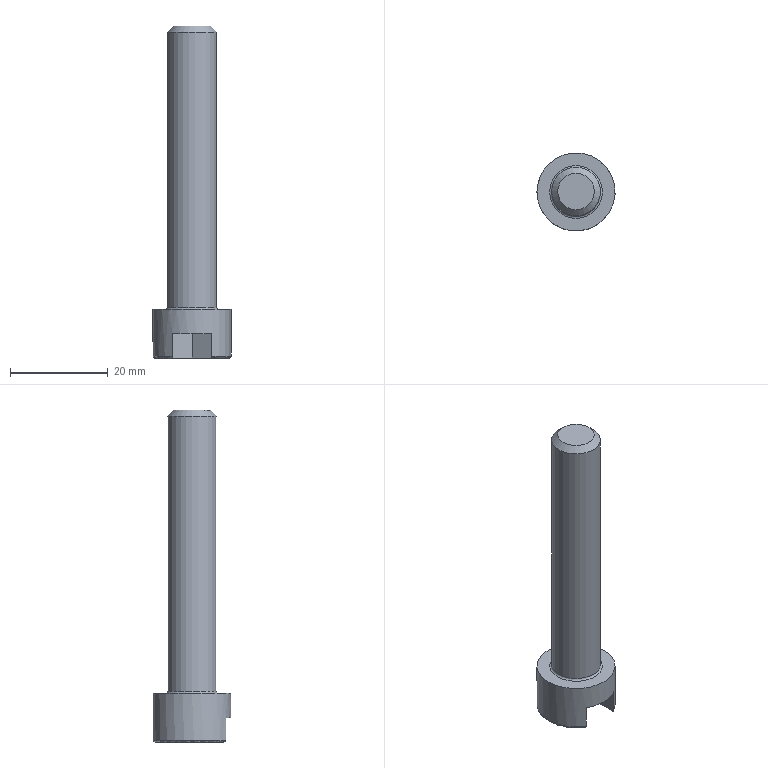Part | STEP file | solid 159 | 1 solid | 13 faces | box 16 x 16 x 68 mm | volume 6098 mm3 | plane 8 | cylinder 2 | torus 2 | cone 1 | commonest cylinder face diameters 10 x1 16 x1